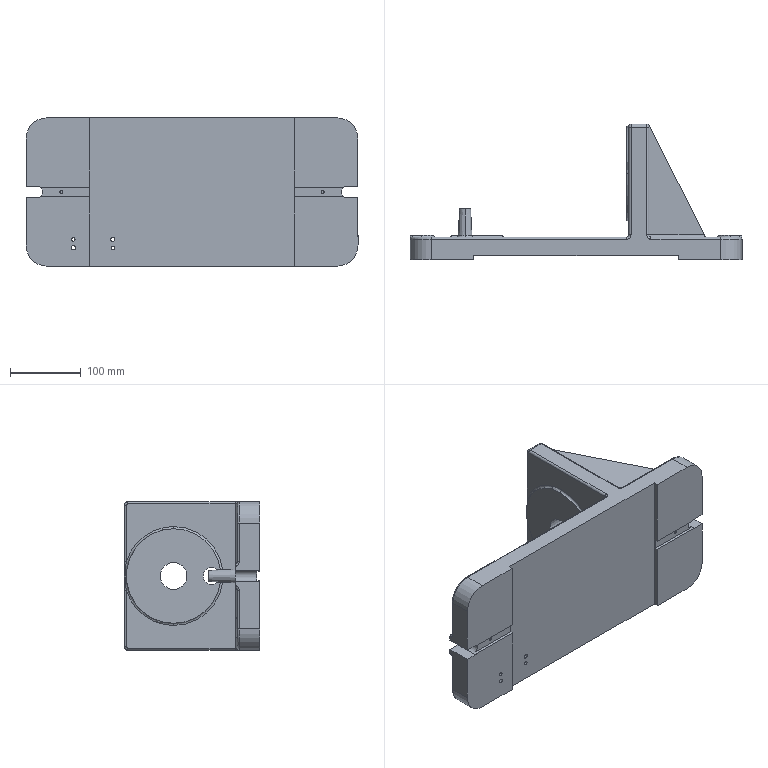Part | SolidWorks | features ICE 10, Fillet 4, Cut 2, Draft 1, Extrusion 1 | 1 solid | 147 faces | box 470 x 192 x 210 mm | volume 3845072 mm3 | cylinder 68 | plane 50 | torus 26 | cone 2 | spline 1 | commonest cylinder face diameters 6 x38 3 x8 4 x4 5 x4 60 x4 8 x2